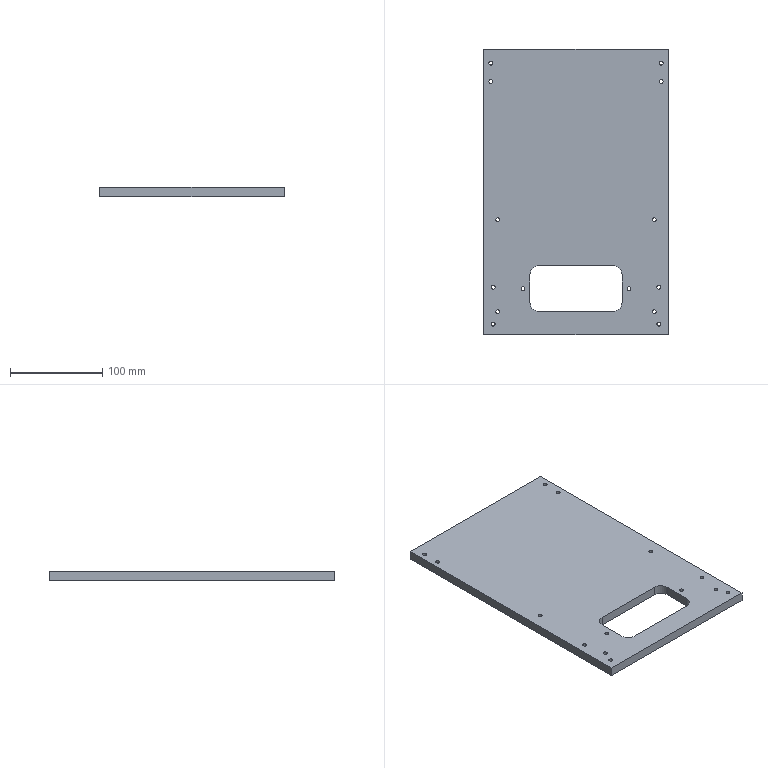Part | SolidWorks | features HoleWzd 4, Cut 1, Extrusion 1, Fillet 1 | 1 solid | 42 faces | box 200 x 310 x 10 mm | volume 568919 mm3 | cylinder 32 | plane 10 | commonest cylinder face diameters 4.2 x28 20 x4
STEP:
#1=CARTESIAN_POINT('',(-87.9,-143.5,5.));
#2=VERTEX_POINT('',#1);
#3=CARTESIAN_POINT('',(-92.1,-143.5,5.));
#4=VERTEX_POINT('',#3);
#5=CARTESIAN_POINT('',(-90.,-143.5,5.));
#6=DIRECTION('',(0.,0.,-1.));
#7=DIRECTION('',(-1.,0.,0.));
#8=AXIS2_PLACEMENT_3D('',#5,#6,#7);
#9=CIRCLE('',#8,2.1);
#10=EDGE_CURVE('',#2,#4,#9,.T.);
#11=ORIENTED_EDGE('',*,*,#10,.F.);
#12=CARTESIAN_POINT('',(-87.9,-143.5,-5.));
#13=VERTEX_POINT('',#12);
#14=CARTESIAN_POINT('',(-87.9,-143.5,-5.));
#15=DIRECTION('',(0.,0.,-1.));
#16=VECTOR('',#15,1000.);
#17=LINE('',#14,#16);
#18=EDGE_CURVE('',#2,#13,#17,.T.);
#19=ORIENTED_EDGE('',*,*,#18,.T.);
#20=CARTESIAN_POINT('',(-92.1,-143.5,-5.));
#21=VERTEX_POINT('',#20);
#22=CARTESIAN_POINT('',(-90.,-143.5,-5.));
#23=DIRECTION('',(0.,0.,-1.));
#24=DIRECTION('',(-1.,0.,0.));
#25=AXIS2_PLACEMENT_3D('',#22,#23,#24);
#26=CIRCLE('',#25,2.1);
#27=EDGE_CURVE('',#13,#21,#26,.T.);
#28=ORIENTED_EDGE('',*,*,#27,.T.);
#29=CARTESIAN_POINT('',(-92.1,-143.5,-5.));
#30=DIRECTION('',(0.,0.,-1.));
#31=VECTOR('',#30,1000.);
#32=LINE('',#29,#31);
#33=EDGE_CURVE('',#4,#21,#32,.T.);
#34=ORIENTED_EDGE('',*,*,#33,.F.);
#35=EDGE_LOOP('',(#11,#19,#28,#34));
#36=FACE_OUTER_BOUND('',#35,.T.);
#37=CARTESIAN_POINT('',(-90.,-143.5,-5.));
#38=DIRECTION('',(0.,0.,-1.));
#39=DIRECTION('',(-1.,0.,0.));
#40=AXIS2_PLACEMENT_3D('',#37,#38,#39);
#41=CYLINDRICAL_SURFACE('',#40,2.1);
#42=ADVANCED_FACE('',(#36),#41,.F.);
#43=CARTESIAN_POINT('',(-87.9,-103.5,5.));
#44=VERTEX_POINT('',#43);
#45=CARTESIAN_POINT('',(-92.1,-103.5,5.));
#46=VERTEX_POINT('',#45);
#47=CARTESIAN_POINT('',(-90.,-103.5,5.));
#48=DIRECTION('',(0.,0.,-1.));
#49=DIRECTION('',(-1.,0.,0.));
#50=AXIS2_PLACEMENT_3D('',#47,#48,#49);
#51=CIRCLE('',#50,2.1);
#52=EDGE_CURVE('',#44,#46,#51,.T.);
#53=ORIENTED_EDGE('',*,*,#52,.F.);
#54=CARTESIAN_POINT('',(-87.9,-103.5,-5.));
#55=VERTEX_POINT('',#54);
#56=CARTESIAN_POINT('',(-87.9,-103.5,-5.));
#57=DIRECTION('',(0.,0.,-1.));
#58=VECTOR('',#57,1000.);
#59=LINE('',#56,#58);
#60=EDGE_CURVE('',#44,#55,#59,.T.);
#61=ORIENTED_EDGE('',*,*,#60,.T.);
#62=CARTESIAN_POINT('',(-92.1,-103.5,-5.));
#63=VERTEX_POINT('',#62);
#64=CARTESIAN_POINT('',(-90.,-103.5,-5.));
#65=DIRECTION('',(0.,0.,-1.));
#66=DIRECTION('',(-1.,0.,0.));
#67=AXIS2_PLACEMENT_3D('',#64,#65,#66);
#68=CIRCLE('',#67,2.1);
#69=EDGE_CURVE('',#55,#63,#68,.T.);
#70=ORIENTED_EDGE('',*,*,#69,.T.);
#71=CARTESIAN_POINT('',(-92.1,-103.5,-5.));
#72=DIRECTION('',(0.,0.,-1.));
#73=VECTOR('',#72,1000.);
#74=LINE('',#71,#73);
#75=EDGE_CURVE('',#46,#63,#74,.T.);
#76=ORIENTED_EDGE('',*,*,#75,.F.);
#77=EDGE_LOOP('',(#53,#61,#70,#76));
#78=FACE_OUTER_BOUND('',#77,.T.);
#79=CARTESIAN_POINT('',(-90.,-103.5,-5.));
#80=DIRECTION('',(0.,0.,-1.));
#81=DIRECTION('',(-1.,0.,0.));
#82=AXIS2_PLACEMENT_3D('',#79,#80,#81);
#83=CYLINDRICAL_SURFACE('',#82,2.1);
#84=ADVANCED_FACE('',(#78),#83,.F.);
#85=CARTESIAN_POINT('',(92.1,-103.5,5.));
#86=VERTEX_POINT('',#85);
#87=CARTESIAN_POINT('',(87.9,-103.5,5.));
#88=VERTEX_POINT('',#87);
#89=CARTESIAN_POINT('',(90.,-103.5,5.));
#90=DIRECTION('',(0.,0.,-1.));
#91=DIRECTION('',(-1.,0.,0.));
#92=AXIS2_PLACEMENT_3D('',#89,#90,#91);
#93=CIRCLE('',#92,2.1);
#94=EDGE_CURVE('',#86,#88,#93,.T.);
#95=ORIENTED_EDGE('',*,*,#94,.F.);
#96=CARTESIAN_POINT('',(92.1,-103.5,-5.));
#97=VERTEX_POINT('',#96);
#98=CARTESIAN_POINT('',(92.1,-103.5,-5.));
#99=DIRECTION('',(0.,0.,-1.));
#100=VECTOR('',#99,1000.);
#101=LINE('',#98,#100);
#102=EDGE_CURVE('',#86,#97,#101,.T.);
#103=ORIENTED_EDGE('',*,*,#102,.T.);
#104=CARTESIAN_POINT('',(87.9,-103.5,-5.));
#105=VERTEX_POINT('',#104);
#106=CARTESIAN_POINT('',(90.,-103.5,-5.));
#107=DIRECTION('',(0.,0.,-1.));
#108=DIRECTION('',(-1.,0.,0.));
#109=AXIS2_PLACEMENT_3D('',#106,#107,#108);
#110=CIRCLE('',#109,2.1);
#111=EDGE_CURVE('',#97,#105,#110,.T.);
#112=ORIENTED_EDGE('',*,*,#111,.T.);
#113=CARTESIAN_POINT('',(87.9,-103.5,-5.));
#114=DIRECTION('',(0.,0.,-1.));
#115=VECTOR('',#114,1000.);
#116=LINE('',#113,#115);
#117=EDGE_CURVE('',#88,#105,#116,.T.);
#118=ORIENTED_EDGE('',*,*,#117,.F.);
#119=EDGE_LOOP('',(#95,#103,#112,#118));
#120=FACE_OUTER_BOUND('',#119,.T.);
#121=CARTESIAN_POINT('',(90.,-103.5,-5.));
#122=DIRECTION('',(0.,0.,-1.));
#123=DIRECTION('',(-1.,0.,0.));
#124=AXIS2_PLACEMENT_3D('',#121,#122,#123);
#125=CYLINDRICAL_SURFACE('',#124,2.1);
#126=ADVANCED_FACE('',(#120),#125,.F.);
#127=CARTESIAN_POINT('',(92.1,-143.5,5.));
#128=VERTEX_POINT('',#127);
#129=CARTESIAN_POINT('',(87.9,-143.5,5.));
#130=VERTEX_POINT('',#129);
#131=CARTESIAN_POINT('',(90.,-143.5,5.));
#132=DIRECTION('',(0.,0.,-1.));
#133=DIRECTION('',(-1.,0.,0.));
#134=AXIS2_PLACEMENT_3D('',#131,#132,#133);
#135=CIRCLE('',#134,2.1);
#136=EDGE_CURVE('',#128,#130,#135,.T.);
#137=ORIENTED_EDGE('',*,*,#136,.F.);
#138=CARTESIAN_POINT('',(92.1,-143.5,-5.));
#139=VERTEX_POINT('',#138);
#140=CARTESIAN_POINT('',(92.1,-143.5,-5.));
#141=DIRECTION('',(0.,0.,-1.));
#142=VECTOR('',#141,1000.);
#143=LINE('',#140,#142);
#144=EDGE_CURVE('',#128,#139,#143,.T.);
#145=ORIENTED_EDGE('',*,*,#144,.T.);
#146=CARTESIAN_POINT('',(87.9,-143.5,-5.));
#147=VERTEX_POINT('',#146);
#148=CARTESIAN_POINT('',(90.,-143.5,-5.));
#149=DIRECTION('',(0.,0.,-1.));
#150=DIRECTION('',(-1.,0.,0.));
#151=AXIS2_PLACEMENT_3D('',#148,#149,#150);
#152=CIRCLE('',#151,2.1);
#153=EDGE_CURVE('',#139,#147,#152,.T.);
#154=ORIENTED_EDGE('',*,*,#153,.T.);
#155=CARTESIAN_POINT('',(87.9,-143.5,-5.));
#156=DIRECTION('',(0.,0.,-1.));
#157=VECTOR('',#156,1000.);
#158=LINE('',#155,#157);
#159=EDGE_CURVE('',#130,#147,#158,.T.);
#160=ORIENTED_EDGE('',*,*,#159,.F.);
#161=EDGE_LOOP('',(#137,#145,#154,#160));
#162=FACE_OUTER_BOUND('',#161,.T.);
#163=CARTESIAN_POINT('',(90.,-143.5,-5.));
#164=DIRECTION('',(0.,0.,-1.));
#165=DIRECTION('',(-1.,0.,0.));
#166=AXIS2_PLACEMENT_3D('',#163,#164,#165);
#167=CYLINDRICAL_SURFACE('',#166,2.1);
#168=ADVANCED_FACE('',(#162),#167,.F.);
#169=CARTESIAN_POINT('',(59.6,-105.,5.));
#170=VERTEX_POINT('',#169);
#171=CARTESIAN_POINT('',(55.4,-105.,5.));
#172=VERTEX_POINT('',#171);
#173=CARTESIAN_POINT('',(57.5,-105.,5.));
#174=DIRECTION('',(0.,0.,-1.));
#175=DIRECTION('',(-1.,0.,0.));
#176=AXIS2_PLACEMENT_3D('',#173,#174,#175);
#177=CIRCLE('',#176,2.1);
#178=EDGE_CURVE('',#170,#172,#177,.T.);
#179=ORIENTED_EDGE('',*,*,#178,.F.);
#180=CARTESIAN_POINT('',(59.6,-105.,-5.));
#181=VERTEX_POINT('',#180);
#182=CARTESIAN_POINT('',(59.6,-105.,-5.));
#183=DIRECTION('',(0.,0.,-1.));
#184=VECTOR('',#183,1000.);
#185=LINE('',#182,#184);
#186=EDGE_CURVE('',#170,#181,#185,.T.);
#187=ORIENTED_EDGE('',*,*,#186,.T.);
#188=CARTESIAN_POINT('',(55.4,-105.,-5.));
#189=VERTEX_POINT('',#188);
#190=CARTESIAN_POINT('',(57.5,-105.,-5.));
#191=DIRECTION('',(0.,0.,-1.));
#192=DIRECTION('',(-1.,0.,0.));
#193=AXIS2_PLACEMENT_3D('',#190,#191,#192);
#194=CIRCLE('',#193,2.1);
#195=EDGE_CURVE('',#181,#189,#194,.T.);
#196=ORIENTED_EDGE('',*,*,#195,.T.);
#197=CARTESIAN_POINT('',(55.4,-105.,-5.));
#198=DIRECTION('',(0.,0.,-1.));
#199=VECTOR('',#198,1000.);
#200=LINE('',#197,#199);
#201=EDGE_CURVE('',#172,#189,#200,.T.);
#202=ORIENTED_EDGE('',*,*,#201,.F.);
#203=EDGE_LOOP('',(#179,#187,#196,#202));
#204=FACE_OUTER_BOUND('',#203,.T.);
#205=CARTESIAN_POINT('',(57.5,-105.,-5.));
#206=DIRECTION('',(0.,0.,-1.));
#207=DIRECTION('',(-1.,0.,0.));
#208=AXIS2_PLACEMENT_3D('',#205,#206,#207);
#209=CYLINDRICAL_SURFACE('',#208,2.1);
#210=ADVANCED_FACE('',(#204),#209,.F.);
#211=CARTESIAN_POINT('',(-55.4,-105.,5.));
#212=VERTEX_POINT('',#211);
#213=CARTESIAN_POINT('',(-59.6,-105.,5.));
#214=VERTEX_POINT('',#213);
#215=CARTESIAN_POINT('',(-57.5,-105.,5.));
#216=DIRECTION('',(0.,0.,-1.));
#217=DIRECTION('',(-1.,0.,0.));
#218=AXIS2_PLACEMENT_3D('',#215,#216,#217);
#219=CIRCLE('',#218,2.1);
#220=EDGE_CURVE('',#212,#214,#219,.T.);
#221=ORIENTED_EDGE('',*,*,#220,.F.);
#222=CARTESIAN_POINT('',(-55.4,-105.,-5.));
#223=VERTEX_POINT('',#222);
#224=CARTESIAN_POINT('',(-55.4,-105.,-5.));
#225=DIRECTION('',(0.,0.,-1.));
#226=VECTOR('',#225,1000.);
#227=LINE('',#224,#226);
#228=EDGE_CURVE('',#212,#223,#227,.T.);
#229=ORIENTED_EDGE('',*,*,#228,.T.);
#230=CARTESIAN_POINT('',(-59.6,-105.,-5.));
#231=VERTEX_POINT('',#230);
#232=CARTESIAN_POINT('',(-57.5,-105.,-5.));
#233=DIRECTION('',(0.,0.,-1.));
#234=DIRECTION('',(-1.,0.,0.));
#235=AXIS2_PLACEMENT_3D('',#232,#233,#234);
#236=CIRCLE('',#235,2.1);
#237=EDGE_CURVE('',#223,#231,#236,.T.);
#238=ORIENTED_EDGE('',*,*,#237,.T.);
#239=CARTESIAN_POINT('',(-59.6,-105.,-5.));
#240=DIRECTION('',(0.,0.,-1.));
#241=VECTOR('',#240,1000.);
#242=LINE('',#239,#241);
#243=EDGE_CURVE('',#214,#231,#242,.T.);
#244=ORIENTED_EDGE('',*,*,#243,.F.);
#245=EDGE_LOOP('',(#221,#229,#238,#244));
#246=FACE_OUTER_BOUND('',#245,.T.);
#247=CARTESIAN_POINT('',(-57.5,-105.,-5.));
#248=DIRECTION('',(0.,0.,-1.));
#249=DIRECTION('',(-1.,0.,0.));
#250=AXIS2_PLACEMENT_3D('',#247,#248,#249);
#251=CYLINDRICAL_SURFACE('',#250,2.1);
#252=ADVANCED_FACE('',(#246),#251,.F.);
#253=CARTESIAN_POINT('',(-90.4,120.,5.));
#254=VERTEX_POINT('',#253);
#255=CARTESIAN_POINT('',(-94.6,120.,5.));
#256=VERTEX_POINT('',#255);
#257=CARTESIAN_POINT('',(-92.5,120.,5.));
#258=DIRECTION('',(0.,0.,-1.));
#259=DIRECTION('',(-1.,0.,0.));
#260=AXIS2_PLACEMENT_3D('',#257,#258,#259);
#261=CIRCLE('',#260,2.1);
#262=EDGE_CURVE('',#254,#256,#261,.T.);
#263=ORIENTED_EDGE('',*,*,#262,.F.);
#264=CARTESIAN_POINT('',(-90.4,120.,-5.));
#265=VERTEX_POINT('',#264);
#266=CARTESIAN_POINT('',(-90.4,120.,-5.));
#267=DIRECTION('',(0.,0.,-1.));
#268=VECTOR('',#267,1000.);
#269=LINE('',#266,#268);
#270=EDGE_CURVE('',#254,#265,#269,.T.);
#271=ORIENTED_EDGE('',*,*,#270,.T.);
#272=CARTESIAN_POINT('',(-94.6,120.,-5.));
#273=VERTEX_POINT('',#272);
#274=CARTESIAN_POINT('',(-92.5,120.,-5.));
#275=DIRECTION('',(0.,0.,-1.));
#276=DIRECTION('',(-1.,0.,0.));
#277=AXIS2_PLACEMENT_3D('',#274,#275,#276);
#278=CIRCLE('',#277,2.1);
#279=EDGE_CURVE('',#265,#273,#278,.T.);
#280=ORIENTED_EDGE('',*,*,#279,.T.);
#281=CARTESIAN_POINT('',(-94.6,120.,-5.));
#282=DIRECTION('',(0.,0.,-1.));
#283=VECTOR('',#282,1000.);
#284=LINE('',#281,#283);
#285=EDGE_CURVE('',#256,#273,#284,.T.);
#286=ORIENTED_EDGE('',*,*,#285,.F.);
#287=EDGE_LOOP('',(#263,#271,#280,#286));
#288=FACE_OUTER_BOUND('',#287,.T.);
#289=CARTESIAN_POINT('',(-92.5,120.,-5.));
#290=DIRECTION('',(0.,0.,-1.));
#291=DIRECTION('',(-1.,0.,0.));
#292=AXIS2_PLACEMENT_3D('',#289,#290,#291);
#293=CYLINDRICAL_SURFACE('',#292,2.1);
#294=ADVANCED_FACE('',(#288),#293,.F.);
#295=CARTESIAN_POINT('',(-90.4,140.,5.));
#296=VERTEX_POINT('',#295);
#297=CARTESIAN_POINT('',(-94.6,140.,5.));
#298=VERTEX_POINT('',#297);
#299=CARTESIAN_POINT('',(-92.5,140.,5.));
#300=DIRECTION('',(0.,0.,-1.));
#301=DIRECTION('',(-1.,0.,0.));
#302=AXIS2_PLACEMENT_3D('',#299,#300,#301);
#303=CIRCLE('',#302,2.1);
#304=EDGE_CURVE('',#296,#298,#303,.T.);
#305=ORIENTED_EDGE('',*,*,#304,.F.);
#306=CARTESIAN_POINT('',(-90.4,140.,-5.));
#307=VERTEX_POINT('',#306);
#308=CARTESIAN_POINT('',(-90.4,140.,-5.));
#309=DIRECTION('',(0.,0.,-1.));
#310=VECTOR('',#309,1000.);
#311=LINE('',#308,#310);
#312=EDGE_CURVE('',#296,#307,#311,.T.);
#313=ORIENTED_EDGE('',*,*,#312,.T.);
#314=CARTESIAN_POINT('',(-94.6,140.,-5.));
#315=VERTEX_POINT('',#314);
#316=CARTESIAN_POINT('',(-92.5,140.,-5.));
#317=DIRECTION('',(0.,0.,-1.));
#318=DIRECTION('',(-1.,0.,0.));
#319=AXIS2_PLACEMENT_3D('',#316,#317,#318);
#320=CIRCLE('',#319,2.1);
#321=EDGE_CURVE('',#307,#315,#320,.T.);
#322=ORIENTED_EDGE('',*,*,#321,.T.);
#323=CARTESIAN_POINT('',(-94.6,140.,-5.));
#324=DIRECTION('',(0.,0.,-1.));
#325=VECTOR('',#324,1000.);
#326=LINE('',#323,#325);
#327=EDGE_CURVE('',#298,#315,#326,.T.);
#328=ORIENTED_EDGE('',*,*,#327,.F.);
#329=EDGE_LOOP('',(#305,#313,#322,#328));
#330=FACE_OUTER_BOUND('',#329,.T.);
#331=CARTESIAN_POINT('',(-92.5,140.,-5.));
#332=DIRECTION('',(0.,0.,-1.));
#333=DIRECTION('',(-1.,0.,0.));
#334=AXIS2_PLACEMENT_3D('',#331,#332,#333);
#335=CYLINDRICAL_SURFACE('',#334,2.1);
#336=ADVANCED_FACE('',(#330),#335,.F.);
#337=CARTESIAN_POINT('',(94.6,140.,5.));
#338=VERTEX_POINT('',#337);
#339=CARTESIAN_POINT('',(90.4,140.,5.));
#340=VERTEX_POINT('',#339);
#341=CARTESIAN_POINT('',(92.5,140.,5.));
#342=DIRECTION('',(0.,0.,-1.));
#343=DIRECTION('',(-1.,0.,0.));
#344=AXIS2_PLACEMENT_3D('',#341,#342,#343);
#345=CIRCLE('',#344,2.1);
#346=EDGE_CURVE('',#338,#340,#345,.T.);
#347=ORIENTED_EDGE('',*,*,#346,.F.);
#348=CARTESIAN_POINT('',(94.6,140.,-5.));
#349=VERTEX_POINT('',#348);
#350=CARTESIAN_POINT('',(94.6,140.,-5.));
#351=DIRECTION('',(0.,0.,-1.));
#352=VECTOR('',#351,1000.);
#353=LINE('',#350,#352);
#354=EDGE_CURVE('',#338,#349,#353,.T.);
#355=ORIENTED_EDGE('',*,*,#354,.T.);
#356=CARTESIAN_POINT('',(90.4,140.,-5.));
#357=VERTEX_POINT('',#356);
#358=CARTESIAN_POINT('',(92.5,140.,-5.));
#359=DIRECTION('',(0.,0.,-1.));
#360=DIRECTION('',(-1.,0.,0.));
#361=AXIS2_PLACEMENT_3D('',#358,#359,#360);
#362=CIRCLE('',#361,2.1);
#363=EDGE_CURVE('',#349,#357,#362,.T.);
#364=ORIENTED_EDGE('',*,*,#363,.T.);
#365=CARTESIAN_POINT('',(90.4,140.,-5.));
#366=DIRECTION('',(0.,0.,-1.));
#367=VECTOR('',#366,1000.);
#368=LINE('',#365,#367);
#369=EDGE_CURVE('',#340,#357,#368,.T.);
#370=ORIENTED_EDGE('',*,*,#369,.F.);
#371=EDGE_LOOP('',(#347,#355,#364,#370));
#372=FACE_OUTER_BOUND('',#371,.T.);
#373=CARTESIAN_POINT('',(92.5,140.,-5.));
#374=DIRECTION('',(0.,0.,-1.));
#375=DIRECTION('',(-1.,0.,0.));
#376=AXIS2_PLACEMENT_3D('',#373,#374,#375);
#377=CYLINDRICAL_SURFACE('',#376,2.1);
#378=ADVANCED_FACE('',(#372),#377,.F.);
#379=CARTESIAN_POINT('',(94.6,120.,5.));
#380=VERTEX_POINT('',#379);
#381=CARTESIAN_POINT('',(90.4,120.,5.));
#382=VERTEX_POINT('',#381);
#383=CARTESIAN_POINT('',(92.5,120.,5.));
#384=DIRECTION('',(0.,0.,-1.));
#385=DIRECTION('',(-1.,0.,0.));
#386=AXIS2_PLACEMENT_3D('',#383,#384,#385);
#387=CIRCLE('',#386,2.1);
#388=EDGE_CURVE('',#380,#382,#387,.T.);
#389=ORIENTED_EDGE('',*,*,#388,.F.);
#390=CARTESIAN_POINT('',(94.6,120.,-5.));
#391=VERTEX_POINT('',#390);
#392=CARTESIAN_POINT('',(94.6,120.,-5.));
#393=DIRECTION('',(0.,0.,-1.));
#394=VECTOR('',#393,1000.);
#395=LINE('',#392,#394);
#396=EDGE_CURVE('',#380,#391,#395,.T.);
#397=ORIENTED_EDGE('',*,*,#396,.T.);
#398=CARTESIAN_POINT('',(90.4,120.,-5.));
#399=VERTEX_POINT('',#398);
#400=CARTESIAN_POINT('',(92.5,120.,-5.));
#401=DIRECTION('',(0.,0.,-1.));
#402=DIRECTION('',(-1.,0.,0.));
#403=AXIS2_PLACEMENT_3D('',#400,#401,#402);
#404=CIRCLE('',#403,2.1);
#405=EDGE_CURVE('',#391,#399,#404,.T.);
#406=ORIENTED_EDGE('',*,*,#405,.T.);
#407=CARTESIAN_POINT('',(90.4,120.,-5.));
#408=DIRECTION('',(0.,0.,-1.));
#409=VECTOR('',#408,1000.);
#410=LINE('',#407,#409);
#411=EDGE_CURVE('',#382,#399,#410,.T.);
#412=ORIENTED_EDGE('',*,*,#411,.F.);
#413=EDGE_LOOP('',(#389,#397,#406,#412));
#414=FACE_OUTER_BOUND('',#413,.T.);
#415=CARTESIAN_POINT('',(92.5,120.,-5.));
#416=DIRECTION('',(0.,0.,-1.));
#417=DIRECTION('',(-1.,0.,0.));
#418=AXIS2_PLACEMENT_3D('',#415,#416,#417);
#419=CYLINDRICAL_SURFACE('',#418,2.1);
#420=ADVANCED_FACE('',(#414),#419,.F.);
#421=CARTESIAN_POINT('',(82.9,-130.,-5.));
#422=VERTEX_POINT('',#421);
#423=CARTESIAN_POINT('',(87.1,-130.,-5.));
#424=VERTEX_POINT('',#423);
#425=CARTESIAN_POINT('',(85.,-130.,-5.));
#426=DIRECTION('',(0.,0.,1.));
#427=DIRECTION('',(1.,0.,0.));
#428=AXIS2_PLACEMENT_3D('',#425,#426,#427);
#429=CIRCLE('',#428,2.1);
#430=EDGE_CURVE('',#422,#424,#429,.T.);
#431=ORIENTED_EDGE('',*,*,#430,.F.);
#432=CARTESIAN_POINT('',(82.9,-130.,5.));
#433=VERTEX_POINT('',#432);
#434=CARTESIAN_POINT('',(82.9,-130.,5.));
#435=DIRECTION('',(0.,0.,1.));
#436=VECTOR('',#435,1000.);
#437=LINE('',#434,#436);
#438=EDGE_CURVE('',#422,#433,#437,.T.);
#439=ORIENTED_EDGE('',*,*,#438,.T.);
#440=CARTESIAN_POINT('',(87.1,-130.,5.));
#441=VERTEX_POINT('',#440);
#442=CARTESIAN_POINT('',(85.,-130.,5.));
#443=DIRECTION('',(0.,0.,1.));
#444=DIRECTION('',(1.,0.,0.));
#445=AXIS2_PLACEMENT_3D('',#442,#443,#444);
#446=CIRCLE('',#445,2.1);
#447=EDGE_CURVE('',#433,#441,#446,.T.);
#448=ORIENTED_EDGE('',*,*,#447,.T.);
#449=CARTESIAN_POINT('',(87.1,-130.,5.));
#450=DIRECTION('',(0.,0.,1.));
#451=VECTOR('',#450,1000.);
#452=LINE('',#449,#451);
#453=EDGE_CURVE('',#424,#441,#452,.T.);
#454=ORIENTED_EDGE('',*,*,#453,.F.);
#455=EDGE_LOOP('',(#431,#439,#448,#454));
#456=FACE_OUTER_BOUND('',#455,.T.);
#457=CARTESIAN_POINT('',(85.,-130.,5.));
#458=DIRECTION('',(0.,0.,1.));
#459=DIRECTION('',(1.,0.,0.));
#460=AXIS2_PLACEMENT_3D('',#457,#458,#459);
#461=CYLINDRICAL_SURFACE('',#460,2.1);
#462=ADVANCED_FACE('',(#456),#461,.F.);
#463=CARTESIAN_POINT('',(82.9,-30.,-5.));
#464=VERTEX_POINT('',#463);
#465=CARTESIAN_POINT('',(87.1,-30.,-5.));
#466=VERTEX_POINT('',#465);
#467=CARTESIAN_POINT('',(85.,-30.,-5.));
#468=DIRECTION('',(0.,0.,1.));
#469=DIRECTION('',(1.,0.,0.));
#470=AXIS2_PLACEMENT_3D('',#467,#468,#469);
#471=CIRCLE('',#470,2.1);
#472=EDGE_CURVE('',#464,#466,#471,.T.);
#473=ORIENTED_EDGE('',*,*,#472,.F.);
#474=CARTESIAN_POINT('',(82.9,-30.,5.));
#475=VERTEX_POINT('',#474);
#476=CARTESIAN_POINT('',(82.9,-30.,5.));
#477=DIRECTION('',(0.,0.,1.));
#478=VECTOR('',#477,1000.);
#479=LINE('',#476,#478);
#480=EDGE_CURVE('',#464,#475,#479,.T.);
#481=ORIENTED_EDGE('',*,*,#480,.T.);
#482=CARTESIAN_POINT('',(87.1,-30.,5.));
#483=VERTEX_POINT('',#482);
#484=CARTESIAN_POINT('',(85.,-30.,5.));
#485=DIRECTION('',(0.,0.,1.));
#486=DIRECTION('',(1.,0.,0.));
#487=AXIS2_PLACEMENT_3D('',#484,#485,#486);
#488=CIRCLE('',#487,2.1);
#489=EDGE_CURVE('',#475,#483,#488,.T.);
#490=ORIENTED_EDGE('',*,*,#489,.T.);
#491=CARTESIAN_POINT('',(87.1,-30.,5.));
#492=DIRECTION('',(0.,0.,1.));
#493=VECTOR('',#492,1000.);
#494=LINE('',#491,#493);
#495=EDGE_CURVE('',#466,#483,#494,.T.);
#496=ORIENTED_EDGE('',*,*,#495,.F.);
#497=EDGE_LOOP('',(#473,#481,#490,#496));
#498=FACE_OUTER_BOUND('',#497,.T.);
#499=CARTESIAN_POINT('',(85.,-30.,5.));
#500=DIRECTION('',(0.,0.,1.));
#501=DIRECTION('',(1.,0.,0.));
#502=AXIS2_PLACEMENT_3D('',#499,#500,#501);
#503=CYLINDRICAL_SURFACE('',#502,2.1);
#504=ADVANCED_FACE('',(#498),#503,.F.);
#505=CARTESIAN_POINT('',(-87.1,-30.,-5.));
#506=VERTEX_POINT('',#505);
#507=CARTESIAN_POINT('',(-82.9,-30.,-5.));
#508=VERTEX_POINT('',#507);
#509=CARTESIAN_POINT('',(-85.,-30.,-5.));
#510=DIRECTION('',(0.,0.,1.));
#511=DIRECTION('',(1.,0.,0.));
#512=AXIS2_PLACEMENT_3D('',#509,#510,#511);
#513=CIRCLE('',#512,2.1);
#514=EDGE_CURVE('',#506,#508,#513,.T.);
#515=ORIENTED_EDGE('',*,*,#514,.F.);
#516=CARTESIAN_POINT('',(-87.1,-30.,5.));
#517=VERTEX_POINT('',#516);
#518=CARTESIAN_POINT('',(-87.1,-30.,5.));
#519=DIRECTION('',(0.,0.,1.));
#520=VECTOR('',#519,1000.);
#521=LINE('',#518,#520);
#522=EDGE_CURVE('',#506,#517,#521,.T.);
#523=ORIENTED_EDGE('',*,*,#522,.T.);
#524=CARTESIAN_POINT('',(-82.9,-30.,5.));
#525=VERTEX_POINT('',#524);
#526=CARTESIAN_POINT('',(-85.,-30.,5.));
#527=DIRECTION('',(0.,0.,1.));
#528=DIRECTION('',(1.,0.,0.));
#529=AXIS2_PLACEMENT_3D('',#526,#527,#528);
#530=CIRCLE('',#529,2.1);
#531=EDGE_CURVE('',#517,#525,#530,.T.);
#532=ORIENTED_EDGE('',*,*,#531,.T.);
#533=CARTESIAN_POINT('',(-82.9,-30.,5.));
#534=DIRECTION('',(0.,0.,1.));
#535=VECTOR('',#534,1000.);
#536=LINE('',#533,#535);
#537=EDGE_CURVE('',#508,#525,#536,.T.);
#538=ORIENTED_EDGE('',*,*,#537,.F.);
#539=EDGE_LOOP('',(#515,#523,#532,#538));
#540=FACE_OUTER_BOUND('',#539,.T.);
#541=CARTESIAN_POINT('',(-85.,-30.,5.));
#542=DIRECTION('',(0.,0.,1.));
#543=DIRECTION('',(1.,0.,0.));
#544=AXIS2_PLACEMENT_3D('',#541,#542,#543);
#545=CYLINDRICAL_SURFACE('',#544,2.1);
#546=ADVANCED_FACE('',(#540),#545,.F.);
#547=CARTESIAN_POINT('',(-87.1,-130.,-5.));
#548=VERTEX_POINT('',#547);
#549=CARTESIAN_POINT('',(-82.9,-130.,-5.));
#550=VERTEX_POINT('',#549);
#551=CARTESIAN_POINT('',(-85.,-130.,-5.));
#552=DIRECTION('',(0.,0.,1.));
#553=DIRECTION('',(1.,0.,0.));
#554=AXIS2_PLACEMENT_3D('',#551,#552,#553);
#555=CIRCLE('',#554,2.1);
#556=EDGE_CURVE('',#548,#550,#555,.T.);
#557=ORIENTED_EDGE('',*,*,#556,.F.);
#558=CARTESIAN_POINT('',(-87.1,-130.,5.));
#559=VERTEX_POINT('',#558);
#560=CARTESIAN_POINT('',(-87.1,-130.,5.));
#561=DIRECTION('',(0.,0.,1.));
#562=VECTOR('',#561,1000.);
#563=LINE('',#560,#562);
#564=EDGE_CURVE('',#548,#559,#563,.T.);
#565=ORIENTED_EDGE('',*,*,#564,.T.);
#566=CARTESIAN_POINT('',(-82.9,-130.,5.));
#567=VERTEX_POINT('',#566);
#568=CARTESIAN_POINT('',(-85.,-130.,5.));
#569=DIRECTION('',(0.,0.,1.));
#570=DIRECTION('',(1.,0.,0.));
#571=AXIS2_PLACEMENT_3D('',#568,#569,#570);
#572=CIRCLE('',#571,2.1);
#573=EDGE_CURVE('',#559,#567,#572,.T.);
#574=ORIENTED_EDGE('',*,*,#573,.T.);
#575=CARTESIAN_POINT('',(-82.9,-130.,5.));
#576=DIRECTION('',(0.,0.,1.));
#577=VECTOR('',#576,1000.);
#578=LINE('',#575,#577);
#579=EDGE_CURVE('',#550,#567,#578,.T.);
#580=ORIENTED_EDGE('',*,*,#579,.F.);
#581=EDGE_LOOP('',(#557,#565,#574,#580));
#582=FACE_OUTER_BOUND('',#581,.T.);
#583=CARTESIAN_POINT('',(-85.,-130.,5.));
#584=DIRECTION('',(0.,0.,1.));
#585=DIRECTION('',(1.,0.,0.));
#586=AXIS2_PLACEMENT_3D('',#583,#584,#585);
#587=CYLINDRICAL_SURFACE('',#586,2.1);
#588=ADVANCED_FACE('',(#582),#587,.F.);
#589=CARTESIAN_POINT('',(100.,-155.,-5.));
#590=VERTEX_POINT('',#589);
#591=CARTESIAN_POINT('',(100.,155.,-5.));
#592=VERTEX_POINT('',#591);
#593=CARTESIAN_POINT('',(100.,-155.,-5.));
#594=DIRECTION('',(0.,1.,0.));
#595=VECTOR('',#594,1000.);
#596=LINE('',#593,#595);
#597=EDGE_CURVE('',#590,#592,#596,.T.);
#598=ORIENTED_EDGE('',*,*,#597,.T.);
#599=CARTESIAN_POINT('',(100.,155.,5.));
#600=VERTEX_POINT('',#599);
#601=CARTESIAN_POINT('',(100.,155.,5.));
#602=DIRECTION('',(0.,0.,-1.));
#603=VECTOR('',#602,1000.);
#604=LINE('',#601,#603);
#605=EDGE_CURVE('',#600,#592,#604,.T.);
#606=ORIENTED_EDGE('',*,*,#605,.F.);
#607=CARTESIAN_POINT('',(100.,-155.,5.));
#608=VERTEX_POINT('',#607);
#609=CARTESIAN_POINT('',(100.,-155.,5.));
#610=DIRECTION('',(0.,1.,0.));
#611=VECTOR('',#610,1000.);
#612=LINE('',#609,#611);
#613=EDGE_CURVE('',#608,#600,#612,.T.);
#614=ORIENTED_EDGE('',*,*,#613,.F.);
#615=CARTESIAN_POINT('',(100.,-155.,5.));
#616=DIRECTION('',(0.,0.,-1.));
#617=VECTOR('',#616,1000.);
#618=LINE('',#615,#617);
#619=EDGE_CURVE('',#608,#590,#618,.T.);
#620=ORIENTED_EDGE('',*,*,#619,.T.);
#621=EDGE_LOOP('',(#598,#606,#614,#620));
#622=FACE_OUTER_BOUND('',#621,.T.);
#623=CARTESIAN_POINT('',(100.,-155.,5.));
#624=DIRECTION('',(-1.,0.,0.));
#625=DIRECTION('',(0.,0.,1.));
#626=AXIS2_PLACEMENT_3D('',#623,#624,#625);
#627=PLANE('',#626);
#628=ADVANCED_FACE('',(#622),#627,.F.);
#629=CARTESIAN_POINT('',(-100.,155.,-5.));
#630=VERTEX_POINT('',#629);
#631=CARTESIAN_POINT('',(-100.,155.,-5.));
#632=DIRECTION('',(-1.,0.,0.));
#633=VECTOR('',#632,1000.);
#634=LINE('',#631,#633);
#635=EDGE_CURVE('',#592,#630,#634,.T.);
#636=ORIENTED_EDGE('',*,*,#635,.T.);
#637=CARTESIAN_POINT('',(-100.,155.,5.));
#638=VERTEX_POINT('',#637);
#639=CARTESIAN_POINT('',(-100.,155.,5.));
#640=DIRECTION('',(0.,0.,-1.));
#641=VECTOR('',#640,1000.);
#642=LINE('',#639,#641);
#643=EDGE_CURVE('',#638,#630,#642,.T.);
#644=ORIENTED_EDGE('',*,*,#643,.F.);
#645=CARTESIAN_POINT('',(-100.,155.,5.));
#646=DIRECTION('',(-1.,0.,0.));
#647=VECTOR('',#646,1000.);
#648=LINE('',#645,#647);
#649=EDGE_CURVE('',#600,#638,#648,.T.);
#650=ORIENTED_EDGE('',*,*,#649,.F.);
#651=ORIENTED_EDGE('',*,*,#605,.T.);
#652=EDGE_LOOP('',(#636,#644,#650,#651));
#653=FACE_OUTER_BOUND('',#652,.T.);
#654=CARTESIAN_POINT('',(-100.,155.,5.));
#655=DIRECTION('',(0.,-1.,0.));
#656=DIRECTION('',(0.,0.,-1.));
#657=AXIS2_PLACEMENT_3D('',#654,#655,#656);
#658=PLANE('',#657);
#659=ADVANCED_FACE('',(#653),#658,.F.);
#660=CARTESIAN_POINT('',(-100.,-155.,-5.));
#661=VERTEX_POINT('',#660);
#662=CARTESIAN_POINT('',(-100.,-155.,-5.));
#663=DIRECTION('',(0.,-1.,0.));
#664=VECTOR('',#663,1000.);
#665=LINE('',#662,#664);
#666=EDGE_CURVE('',#630,#661,#665,.T.);
#667=ORIENTED_EDGE('',*,*,#666,.T.);
#668=CARTESIAN_POINT('',(-100.,-155.,5.));
#669=VERTEX_POINT('',#668);
#670=CARTESIAN_POINT('',(-100.,-155.,5.));
#671=DIRECTION('',(0.,0.,-1.));
#672=VECTOR('',#671,1000.);
#673=LINE('',#670,#672);
#674=EDGE_CURVE('',#669,#661,#673,.T.);
#675=ORIENTED_EDGE('',*,*,#674,.F.);
#676=CARTESIAN_POINT('',(-100.,-155.,5.));
#677=DIRECTION('',(0.,-1.,0.));
#678=VECTOR('',#677,1000.);
#679=LINE('',#676,#678);
#680=EDGE_CURVE('',#638,#669,#679,.T.);
#681=ORIENTED_EDGE('',*,*,#680,.F.);
#682=ORIENTED_EDGE('',*,*,#643,.T.);
#683=EDGE_LOOP('',(#667,#675,#681,#682));
#684=FACE_OUTER_BOUND('',#683,.T.);
#685=CARTESIAN_POINT('',(-100.,-155.,5.));
#686=DIRECTION('',(1.,0.,0.));
#687=DIRECTION('',(0.,0.,-1.));
#688=AXIS2_PLACEMENT_3D('',#685,#686,#687);
#689=PLANE('',#688);
#690=ADVANCED_FACE('',(#684),#689,.F.);
#691=CARTESIAN_POINT('',(-100.,-155.,-5.));
#692=DIRECTION('',(1.,0.,0.));
#693=VECTOR('',#692,1000.);
#694=LINE('',#691,#693);
#695=EDGE_CURVE('',#661,#590,#694,.T.);
#696=ORIENTED_EDGE('',*,*,#695,.T.);
#697=ORIENTED_EDGE('',*,*,#619,.F.);
#698=CARTESIAN_POINT('',(-100.,-155.,5.));
#699=DIRECTION('',(1.,0.,0.));
#700=VECTOR('',#699,1000.);
#701=LINE('',#698,#700);
#702=EDGE_CURVE('',#669,#608,#701,.T.);
#703=ORIENTED_EDGE('',*,*,#702,.F.);
#704=ORIENTED_EDGE('',*,*,#674,.T.);
#705=EDGE_LOOP('',(#696,#697,#703,#704));
#706=FACE_OUTER_BOUND('',#705,.T.);
#707=CARTESIAN_POINT('',(-100.,-155.,5.));
#708=DIRECTION('',(0.,1.,0.));
#709=DIRECTION('',(0.,0.,1.));
#710=AXIS2_PLACEMENT_3D('',#707,#708,#709);
#711=PLANE('',#710);
#712=ADVANCED_FACE('',(#706),#711,.F.);
#713=CARTESIAN_POINT('',(-90.,-143.5,5.));
#714=DIRECTION('',(0.,0.,-1.));
#715=DIRECTION('',(-1.,0.,0.));
#716=AXIS2_PLACEMENT_3D('',#713,#714,#715);
#717=CIRCLE('',#716,2.1);
#718=EDGE_CURVE('',#4,#2,#717,.T.);
#719=ORIENTED_EDGE('',*,*,#718,.T.);
#720=ORIENTED_EDGE('',*,*,#10,.T.);
#721=EDGE_LOOP('',(#719,#720));
#722=FACE_BOUND('',#721,.T.);
#723=CARTESIAN_POINT('',(-90.,-103.5,5.));
#724=DIRECTION('',(0.,0.,-1.));
#725=DIRECTION('',(-1.,0.,0.));
#726=AXIS2_PLACEMENT_3D('',#723,#724,#725);
#727=CIRCLE('',#726,2.1);
#728=EDGE_CURVE('',#46,#44,#727,.T.);
#729=ORIENTED_EDGE('',*,*,#728,.T.);
#730=ORIENTED_EDGE('',*,*,#52,.T.);
#731=EDGE_LOOP('',(#729,#730));
#732=FACE_BOUND('',#731,.T.);
#733=CARTESIAN_POINT('',(90.,-103.5,5.));
#734=DIRECTION('',(0.,0.,-1.));
#735=DIRECTION('',(-1.,0.,0.));
#736=AXIS2_PLACEMENT_3D('',#733,#734,#735);
#737=CIRCLE('',#736,2.1);
#738=EDGE_CURVE('',#88,#86,#737,.T.);
#739=ORIENTED_EDGE('',*,*,#738,.T.);
#740=ORIENTED_EDGE('',*,*,#94,.T.);
#741=EDGE_LOOP('',(#739,#740));
#742=FACE_BOUND('',#741,.T.);
#743=CARTESIAN_POINT('',(90.,-143.5,5.));
#744=DIRECTION('',(0.,0.,-1.));
#745=DIRECTION('',(-1.,0.,0.));
#746=AXIS2_PLACEMENT_3D('',#743,#744,#745);
#747=CIRCLE('',#746,2.1);
#748=EDGE_CURVE('',#130,#128,#747,.T.);
#749=ORIENTED_EDGE('',*,*,#748,.T.);
#750=ORIENTED_EDGE('',*,*,#136,.T.);
#751=EDGE_LOOP('',(#749,#750));
#752=FACE_BOUND('',#751,.T.);
#753=CARTESIAN_POINT('',(57.5,-105.,5.));
#754=DIRECTION('',(0.,0.,-1.));
#755=DIRECTION('',(-1.,0.,0.));
#756=AXIS2_PLACEMENT_3D('',#753,#754,#755);
#757=CIRCLE('',#756,2.1);
#758=EDGE_CURVE('',#172,#170,#757,.T.);
#759=ORIENTED_EDGE('',*,*,#758,.T.);
#760=ORIENTED_EDGE('',*,*,#178,.T.);
#761=EDGE_LOOP('',(#759,#760));
#762=FACE_BOUND('',#761,.T.);
#763=CARTESIAN_POINT('',(-57.5,-105.,5.));
#764=DIRECTION('',(0.,0.,-1.));
#765=DIRECTION('',(-1.,0.,0.));
#766=AXIS2_PLACEMENT_3D('',#763,#764,#765);
#767=CIRCLE('',#766,2.1);
#768=EDGE_CURVE('',#214,#212,#767,.T.);
#769=ORIENTED_EDGE('',*,*,#768,.T.);
#770=ORIENTED_EDGE('',*,*,#220,.T.);
#771=EDGE_LOOP('',(#769,#770));
#772=FACE_BOUND('',#771,.T.);
#773=CARTESIAN_POINT('',(-92.5,120.,5.));
#774=DIRECTION('',(0.,0.,-1.));
#775=DIRECTION('',(-1.,0.,0.));
#776=AXIS2_PLACEMENT_3D('',#773,#774,#775);
#777=CIRCLE('',#776,2.1);
#778=EDGE_CURVE('',#256,#254,#777,.T.);
#779=ORIENTED_EDGE('',*,*,#778,.T.);
#780=ORIENTED_EDGE('',*,*,#262,.T.);
#781=EDGE_LOOP('',(#779,#780));
#782=FACE_BOUND('',#781,.T.);
#783=CARTESIAN_POINT('',(-92.5,140.,5.));
#784=DIRECTION('',(0.,0.,-1.));
#785=DIRECTION('',(-1.,0.,0.));
#786=AXIS2_PLACEMENT_3D('',#783,#784,#785);
#787=CIRCLE('',#786,2.1);
#788=EDGE_CURVE('',#298,#296,#787,.T.);
#789=ORIENTED_EDGE('',*,*,#788,.T.);
#790=ORIENTED_EDGE('',*,*,#304,.T.);
#791=EDGE_LOOP('',(#789,#790));
#792=FACE_BOUND('',#791,.T.);
#793=CARTESIAN_POINT('',(92.5,140.,5.));
#794=DIRECTION('',(0.,0.,-1.));
#795=DIRECTION('',(-1.,0.,0.));
#796=AXIS2_PLACEMENT_3D('',#793,#794,#795);
#797=CIRCLE('',#796,2.1);
#798=EDGE_CURVE('',#340,#338,#797,.T.);
#799=ORIENTED_EDGE('',*,*,#798,.T.);
#800=ORIENTED_EDGE('',*,*,#346,.T.);
#801=EDGE_LOOP('',(#799,#800));
#802=FACE_BOUND('',#801,.T.);
#803=CARTESIAN_POINT('',(92.5,120.,5.));
#804=DIRECTION('',(0.,0.,-1.));
#805=DIRECTION('',(-1.,0.,0.));
#806=AXIS2_PLACEMENT_3D('',#803,#804,#805);
#807=CIRCLE('',#806,2.1);
#808=EDGE_CURVE('',#382,#380,#807,.T.);
#809=ORIENTED_EDGE('',*,*,#808,.T.);
#810=ORIENTED_EDGE('',*,*,#388,.T.);
#811=EDGE_LOOP('',(#809,#810));
#812=FACE_BOUND('',#811,.T.);
#813=CARTESIAN_POINT('',(85.,-130.,5.));
#814=DIRECTION('',(0.,0.,1.));
#815=DIRECTION('',(1.,0.,0.));
#816=AXIS2_PLACEMENT_3D('',#813,#814,#815);
#817=CIRCLE('',#816,2.1);
#818=EDGE_CURVE('',#441,#433,#817,.T.);
#819=ORIENTED_EDGE('',*,*,#818,.F.);
#820=ORIENTED_EDGE('',*,*,#447,.F.);
#821=EDGE_LOOP('',(#819,#820));
#822=FACE_BOUND('',#821,.T.);
#823=CARTESIAN_POINT('',(85.,-30.,5.));
#824=DIRECTION('',(0.,0.,1.));
#825=DIRECTION('',(1.,0.,0.));
#826=AXIS2_PLACEMENT_3D('',#823,#824,#825);
#827=CIRCLE('',#826,2.1);
#828=EDGE_CURVE('',#483,#475,#827,.T.);
#829=ORIENTED_EDGE('',*,*,#828,.F.);
#830=ORIENTED_EDGE('',*,*,#489,.F.);
#831=EDGE_LOOP('',(#829,#830));
#832=FACE_BOUND('',#831,.T.);
#833=CARTESIAN_POINT('',(-85.,-30.,5.));
#834=DIRECTION('',(0.,0.,1.));
#835=DIRECTION('',(1.,0.,0.));
#836=AXIS2_PLACEMENT_3D('',#833,#834,#835);
#837=CIRCLE('',#836,2.1);
#838=EDGE_CURVE('',#525,#517,#837,.T.);
#839=ORIENTED_EDGE('',*,*,#838,.F.);
#840=ORIENTED_EDGE('',*,*,#531,.F.);
#841=EDGE_LOOP('',(#839,#840));
#842=FACE_BOUND('',#841,.T.);
#843=CARTESIAN_POINT('',(-85.,-130.,5.));
#844=DIRECTION('',(0.,0.,1.));
#845=DIRECTION('',(1.,0.,0.));
#846=AXIS2_PLACEMENT_3D('',#843,#844,#845);
#847=CIRCLE('',#846,2.1);
#848=EDGE_CURVE('',#567,#559,#847,.T.);
#849=ORIENTED_EDGE('',*,*,#848,.F.);
#850=ORIENTED_EDGE('',*,*,#573,.F.);
#851=EDGE_LOOP('',(#849,#850));
#852=FACE_BOUND('',#851,.T.);
#853=CARTESIAN_POINT('',(40.,-80.,5.));
#854=VERTEX_POINT('',#853);
#855=CARTESIAN_POINT('',(-40.,-80.,5.));
#856=VERTEX_POINT('',#855);
#857=CARTESIAN_POINT('',(50.,-80.,5.));
#858=DIRECTION('',(-1.,0.,0.));
#859=VECTOR('',#858,1000.);
#860=LINE('',#857,#859);
#861=EDGE_CURVE('',#854,#856,#860,.T.);
#862=ORIENTED_EDGE('',*,*,#861,.F.);
#863=CARTESIAN_POINT('',(50.,-90.,5.));
#864=VERTEX_POINT('',#863);
#865=CARTESIAN_POINT('',(40.,-90.,5.));
#866=DIRECTION('',(0.,0.,-1.));
#867=DIRECTION('',(-1.,0.,0.));
#868=AXIS2_PLACEMENT_3D('',#865,#866,#867);
#869=CIRCLE('',#868,10.);
#870=EDGE_CURVE('',#854,#864,#869,.T.);
#871=ORIENTED_EDGE('',*,*,#870,.T.);
#872=CARTESIAN_POINT('',(50.,-120.,5.));
#873=VERTEX_POINT('',#872);
#874=CARTESIAN_POINT('',(50.,-130.,5.));
#875=DIRECTION('',(0.,1.,0.));
#876=VECTOR('',#875,1000.);
#877=LINE('',#874,#876);
#878=EDGE_CURVE('',#873,#864,#877,.T.);
#879=ORIENTED_EDGE('',*,*,#878,.F.);
#880=CARTESIAN_POINT('',(40.,-130.,5.));
#881=VERTEX_POINT('',#880);
#882=CARTESIAN_POINT('',(40.,-120.,5.));
#883=DIRECTION('',(0.,0.,-1.));
#884=DIRECTION('',(-1.,0.,0.));
#885=AXIS2_PLACEMENT_3D('',#882,#883,#884);
#886=CIRCLE('',#885,10.);
#887=EDGE_CURVE('',#873,#881,#886,.T.);
#888=ORIENTED_EDGE('',*,*,#887,.T.);
#889=CARTESIAN_POINT('',(-40.,-130.,5.));
#890=VERTEX_POINT('',#889);
#891=CARTESIAN_POINT('',(50.,-130.,5.));
#892=DIRECTION('',(1.,0.,0.));
#893=VECTOR('',#892,1000.);
#894=LINE('',#891,#893);
#895=EDGE_CURVE('',#890,#881,#894,.T.);
#896=ORIENTED_EDGE('',*,*,#895,.F.);
#897=CARTESIAN_POINT('',(-50.,-120.,5.));
#898=VERTEX_POINT('',#897);
#899=CARTESIAN_POINT('',(-40.,-120.,5.));
#900=DIRECTION('',(0.,0.,-1.));
#901=DIRECTION('',(-1.,0.,0.));
#902=AXIS2_PLACEMENT_3D('',#899,#900,#901);
#903=CIRCLE('',#902,10.);
#904=EDGE_CURVE('',#890,#898,#903,.T.);
#905=ORIENTED_EDGE('',*,*,#904,.T.);
#906=CARTESIAN_POINT('',(-50.,-90.,5.));
#907=VERTEX_POINT('',#906);
#908=CARTESIAN_POINT('',(-50.,-130.,5.));
#909=DIRECTION('',(0.,-1.,0.));
#910=VECTOR('',#909,1000.);
#911=LINE('',#908,#910);
#912=EDGE_CURVE('',#907,#898,#911,.T.);
#913=ORIENTED_EDGE('',*,*,#912,.F.);
#914=CARTESIAN_POINT('',(-40.,-90.,5.));
#915=DIRECTION('',(0.,0.,-1.));
#916=DIRECTION('',(-1.,0.,0.));
#917=AXIS2_PLACEMENT_3D('',#914,#915,#916);
#918=CIRCLE('',#917,10.);
#919=EDGE_CURVE('',#907,#856,#918,.T.);
#920=ORIENTED_EDGE('',*,*,#919,.T.);
#921=EDGE_LOOP('',(#862,#871,#879,#888,#896,#905,#913,#920));
#922=FACE_BOUND('',#921,.T.);
#923=ORIENTED_EDGE('',*,*,#613,.T.);
#924=ORIENTED_EDGE('',*,*,#649,.T.);
#925=ORIENTED_EDGE('',*,*,#680,.T.);
#926=ORIENTED_EDGE('',*,*,#702,.T.);
#927=EDGE_LOOP('',(#923,#924,#925,#926));
#928=FACE_OUTER_BOUND('',#927,.T.);
#929=CARTESIAN_POINT('',(0.,0.,5.));
#930=DIRECTION('',(0.,0.,-1.));
#931=DIRECTION('',(-1.,0.,0.));
#932=AXIS2_PLACEMENT_3D('',#929,#930,#931);
#933=PLANE('',#932);
#934=ADVANCED_FACE('',(#722,#732,#742,#752,#762,#772,#782,#792,#802,#812,#822,#832,#842,#852,#922,#928),#933,.F.);
#935=CARTESIAN_POINT('',(-90.,-143.5,-5.));
#936=DIRECTION('',(0.,0.,-1.));
#937=DIRECTION('',(-1.,0.,0.));
#938=AXIS2_PLACEMENT_3D('',#935,#936,#937);
#939=CIRCLE('',#938,2.1);
#940=EDGE_CURVE('',#21,#13,#939,.T.);
#941=ORIENTED_EDGE('',*,*,#940,.F.);
#942=ORIENTED_EDGE('',*,*,#27,.F.);
#943=EDGE_LOOP('',(#941,#942));
#944=FACE_BOUND('',#943,.T.);
#945=CARTESIAN_POINT('',(-90.,-103.5,-5.));
#946=DIRECTION('',(0.,0.,-1.));
#947=DIRECTION('',(-1.,0.,0.));
#948=AXIS2_PLACEMENT_3D('',#945,#946,#947);
#949=CIRCLE('',#948,2.1);
#950=EDGE_CURVE('',#63,#55,#949,.T.);
#951=ORIENTED_EDGE('',*,*,#950,.F.);
#952=ORIENTED_EDGE('',*,*,#69,.F.);
#953=EDGE_LOOP('',(#951,#952));
#954=FACE_BOUND('',#953,.T.);
#955=CARTESIAN_POINT('',(90.,-103.5,-5.));
#956=DIRECTION('',(0.,0.,-1.));
#957=DIRECTION('',(-1.,0.,0.));
#958=AXIS2_PLACEMENT_3D('',#955,#956,#957);
#959=CIRCLE('',#958,2.1);
#960=EDGE_CURVE('',#105,#97,#959,.T.);
#961=ORIENTED_EDGE('',*,*,#960,.F.);
#962=ORIENTED_EDGE('',*,*,#111,.F.);
#963=EDGE_LOOP('',(#961,#962));
#964=FACE_BOUND('',#963,.T.);
#965=CARTESIAN_POINT('',(90.,-143.5,-5.));
#966=DIRECTION('',(0.,0.,-1.));
#967=DIRECTION('',(-1.,0.,0.));
#968=AXIS2_PLACEMENT_3D('',#965,#966,#967);
#969=CIRCLE('',#968,2.1);
#970=EDGE_CURVE('',#147,#139,#969,.T.);
#971=ORIENTED_EDGE('',*,*,#970,.F.);
#972=ORIENTED_EDGE('',*,*,#153,.F.);
#973=EDGE_LOOP('',(#971,#972));
#974=FACE_BOUND('',#973,.T.);
#975=CARTESIAN_POINT('',(57.5,-105.,-5.));
#976=DIRECTION('',(0.,0.,-1.));
#977=DIRECTION('',(-1.,0.,0.));
#978=AXIS2_PLACEMENT_3D('',#975,#976,#977);
#979=CIRCLE('',#978,2.1);
#980=EDGE_CURVE('',#189,#181,#979,.T.);
#981=ORIENTED_EDGE('',*,*,#980,.F.);
#982=ORIENTED_EDGE('',*,*,#195,.F.);
#983=EDGE_LOOP('',(#981,#982));
#984=FACE_BOUND('',#983,.T.);
#985=CARTESIAN_POINT('',(-57.5,-105.,-5.));
#986=DIRECTION('',(0.,0.,-1.));
#987=DIRECTION('',(-1.,0.,0.));
#988=AXIS2_PLACEMENT_3D('',#985,#986,#987);
#989=CIRCLE('',#988,2.1);
#990=EDGE_CURVE('',#231,#223,#989,.T.);
#991=ORIENTED_EDGE('',*,*,#990,.F.);
#992=ORIENTED_EDGE('',*,*,#237,.F.);
#993=EDGE_LOOP('',(#991,#992));
#994=FACE_BOUND('',#993,.T.);
#995=CARTESIAN_POINT('',(-92.5,120.,-5.));
#996=DIRECTION('',(0.,0.,-1.));
#997=DIRECTION('',(-1.,0.,0.));
#998=AXIS2_PLACEMENT_3D('',#995,#996,#997);
#999=CIRCLE('',#998,2.1);
#1000=EDGE_CURVE('',#273,#265,#999,.T.);
#1001=ORIENTED_EDGE('',*,*,#1000,.F.);
#1002=ORIENTED_EDGE('',*,*,#279,.F.);
#1003=EDGE_LOOP('',(#1001,#1002));
#1004=FACE_BOUND('',#1003,.T.);
#1005=CARTESIAN_POINT('',(-92.5,140.,-5.));
#1006=DIRECTION('',(0.,0.,-1.));
#1007=DIRECTION('',(-1.,0.,0.));
#1008=AXIS2_PLACEMENT_3D('',#1005,#1006,#1007);
#1009=CIRCLE('',#1008,2.1);
#1010=EDGE_CURVE('',#315,#307,#1009,.T.);
#1011=ORIENTED_EDGE('',*,*,#1010,.F.);
#1012=ORIENTED_EDGE('',*,*,#321,.F.);
#1013=EDGE_LOOP('',(#1011,#1012));
#1014=FACE_BOUND('',#1013,.T.);
#1015=CARTESIAN_POINT('',(92.5,140.,-5.));
#1016=DIRECTION('',(0.,0.,-1.));
#1017=DIRECTION('',(-1.,0.,0.));
#1018=AXIS2_PLACEMENT_3D('',#1015,#1016,#1017);
#1019=CIRCLE('',#1018,2.1);
#1020=EDGE_CURVE('',#357,#349,#1019,.T.);
#1021=ORIENTED_EDGE('',*,*,#1020,.F.);
#1022=ORIENTED_EDGE('',*,*,#363,.F.);
#1023=EDGE_LOOP('',(#1021,#1022));
#1024=FACE_BOUND('',#1023,.T.);
#1025=CARTESIAN_POINT('',(92.5,120.,-5.));
#1026=DIRECTION('',(0.,0.,-1.));
#1027=DIRECTION('',(-1.,0.,0.));
#1028=AXIS2_PLACEMENT_3D('',#1025,#1026,#1027);
#1029=CIRCLE('',#1028,2.1);
#1030=EDGE_CURVE('',#399,#391,#1029,.T.);
#1031=ORIENTED_EDGE('',*,*,#1030,.F.);
#1032=ORIENTED_EDGE('',*,*,#405,.F.);
#1033=EDGE_LOOP('',(#1031,#1032));
#1034=FACE_BOUND('',#1033,.T.);
#1035=CARTESIAN_POINT('',(85.,-130.,-5.));
#1036=DIRECTION('',(0.,0.,1.));
#1037=DIRECTION('',(1.,0.,0.));
#1038=AXIS2_PLACEMENT_3D('',#1035,#1036,#1037);
#1039=CIRCLE('',#1038,2.1);
#1040=EDGE_CURVE('',#424,#422,#1039,.T.);
#1041=ORIENTED_EDGE('',*,*,#1040,.T.);
#1042=ORIENTED_EDGE('',*,*,#430,.T.);
#1043=EDGE_LOOP('',(#1041,#1042));
#1044=FACE_BOUND('',#1043,.T.);
#1045=CARTESIAN_POINT('',(85.,-30.,-5.));
#1046=DIRECTION('',(0.,0.,1.));
#1047=DIRECTION('',(1.,0.,0.));
#1048=AXIS2_PLACEMENT_3D('',#1045,#1046,#1047);
#1049=CIRCLE('',#1048,2.1);
#1050=EDGE_CURVE('',#466,#464,#1049,.T.);
#1051=ORIENTED_EDGE('',*,*,#1050,.T.);
#1052=ORIENTED_EDGE('',*,*,#472,.T.);
#1053=EDGE_LOOP('',(#1051,#1052));
#1054=FACE_BOUND('',#1053,.T.);
#1055=CARTESIAN_POINT('',(-85.,-30.,-5.));
#1056=DIRECTION('',(0.,0.,1.));
#1057=DIRECTION('',(1.,0.,0.));
#1058=AXIS2_PLACEMENT_3D('',#1055,#1056,#1057);
#1059=CIRCLE('',#1058,2.1);
#1060=EDGE_CURVE('',#508,#506,#1059,.T.);
#1061=ORIENTED_EDGE('',*,*,#1060,.T.);
#1062=ORIENTED_EDGE('',*,*,#514,.T.);
#1063=EDGE_LOOP('',(#1061,#1062));
#1064=FACE_BOUND('',#1063,.T.);
#1065=CARTESIAN_POINT('',(-85.,-130.,-5.));
#1066=DIRECTION('',(0.,0.,1.));
#1067=DIRECTION('',(1.,0.,0.));
#1068=AXIS2_PLACEMENT_3D('',#1065,#1066,#1067);
#1069=CIRCLE('',#1068,2.1);
#1070=EDGE_CURVE('',#550,#548,#1069,.T.);
#1071=ORIENTED_EDGE('',*,*,#1070,.T.);
#1072=ORIENTED_EDGE('',*,*,#556,.T.);
#1073=EDGE_LOOP('',(#1071,#1072));
#1074=FACE_BOUND('',#1073,.T.);
#1075=CARTESIAN_POINT('',(-40.,-130.,-5.));
#1076=VERTEX_POINT('',#1075);
#1077=CARTESIAN_POINT('',(40.,-130.,-5.));
#1078=VERTEX_POINT('',#1077);
#1079=CARTESIAN_POINT('',(50.,-130.,-5.));
#1080=DIRECTION('',(1.,0.,0.));
#1081=VECTOR('',#1080,1000.);
#1082=LINE('',#1079,#1081);
#1083=EDGE_CURVE('',#1076,#1078,#1082,.T.);
#1084=ORIENTED_EDGE('',*,*,#1083,.T.);
#1085=CARTESIAN_POINT('',(50.,-120.,-5.));
#1086=VERTEX_POINT('',#1085);
#1087=CARTESIAN_POINT('',(40.,-120.,-5.));
#1088=DIRECTION('',(0.,0.,1.));
#1089=DIRECTION('',(-1.,0.,0.));
#1090=AXIS2_PLACEMENT_3D('',#1087,#1088,#1089);
#1091=CIRCLE('',#1090,10.);
#1092=EDGE_CURVE('',#1078,#1086,#1091,.T.);
#1093=ORIENTED_EDGE('',*,*,#1092,.T.);
#1094=CARTESIAN_POINT('',(50.,-90.,-5.));
#1095=VERTEX_POINT('',#1094);
#1096=CARTESIAN_POINT('',(50.,-130.,-5.));
#1097=DIRECTION('',(0.,1.,0.));
#1098=VECTOR('',#1097,1000.);
#1099=LINE('',#1096,#1098);
#1100=EDGE_CURVE('',#1086,#1095,#1099,.T.);
#1101=ORIENTED_EDGE('',*,*,#1100,.T.);
#1102=CARTESIAN_POINT('',(40.,-80.,-5.));
#1103=VERTEX_POINT('',#1102);
#1104=CARTESIAN_POINT('',(40.,-90.,-5.));
#1105=DIRECTION('',(0.,0.,1.));
#1106=DIRECTION('',(-1.,0.,0.));
#1107=AXIS2_PLACEMENT_3D('',#1104,#1105,#1106);
#1108=CIRCLE('',#1107,10.);
#1109=EDGE_CURVE('',#1095,#1103,#1108,.T.);
#1110=ORIENTED_EDGE('',*,*,#1109,.T.);
#1111=CARTESIAN_POINT('',(-40.,-80.,-5.));
#1112=VERTEX_POINT('',#1111);
#1113=CARTESIAN_POINT('',(50.,-80.,-5.));
#1114=DIRECTION('',(-1.,0.,0.));
#1115=VECTOR('',#1114,1000.);
#1116=LINE('',#1113,#1115);
#1117=EDGE_CURVE('',#1103,#1112,#1116,.T.);
#1118=ORIENTED_EDGE('',*,*,#1117,.T.);
#1119=CARTESIAN_POINT('',(-50.,-90.,-5.));
#1120=VERTEX_POINT('',#1119);
#1121=CARTESIAN_POINT('',(-40.,-90.,-5.));
#1122=DIRECTION('',(0.,0.,1.));
#1123=DIRECTION('',(-1.,0.,0.));
#1124=AXIS2_PLACEMENT_3D('',#1121,#1122,#1123);
#1125=CIRCLE('',#1124,10.);
#1126=EDGE_CURVE('',#1112,#1120,#1125,.T.);
#1127=ORIENTED_EDGE('',*,*,#1126,.T.);
#1128=CARTESIAN_POINT('',(-50.,-120.,-5.));
#1129=VERTEX_POINT('',#1128);
#1130=CARTESIAN_POINT('',(-50.,-130.,-5.));
#1131=DIRECTION('',(0.,-1.,0.));
#1132=VECTOR('',#1131,1000.);
#1133=LINE('',#1130,#1132);
#1134=EDGE_CURVE('',#1120,#1129,#1133,.T.);
#1135=ORIENTED_EDGE('',*,*,#1134,.T.);
#1136=CARTESIAN_POINT('',(-40.,-120.,-5.));
#1137=DIRECTION('',(0.,0.,1.));
#1138=DIRECTION('',(-1.,0.,0.));
#1139=AXIS2_PLACEMENT_3D('',#1136,#1137,#1138);
#1140=CIRCLE('',#1139,10.);
#1141=EDGE_CURVE('',#1129,#1076,#1140,.T.);
#1142=ORIENTED_EDGE('',*,*,#1141,.T.);
#1143=EDGE_LOOP('',(#1084,#1093,#1101,#1110,#1118,#1127,#1135,#1142));
#1144=FACE_BOUND('',#1143,.T.);
#1145=ORIENTED_EDGE('',*,*,#597,.F.);
#1146=ORIENTED_EDGE('',*,*,#695,.F.);
#1147=ORIENTED_EDGE('',*,*,#666,.F.);
#1148=ORIENTED_EDGE('',*,*,#635,.F.);
#1149=EDGE_LOOP('',(#1145,#1146,#1147,#1148));
#1150=FACE_OUTER_BOUND('',#1149,.T.);
#1151=CARTESIAN_POINT('',(0.,0.,-5.));
#1152=DIRECTION('',(0.,0.,-1.));
#1153=DIRECTION('',(-1.,0.,0.));
#1154=AXIS2_PLACEMENT_3D('',#1151,#1152,#1153);
#1155=PLANE('',#1154);
#1156=ADVANCED_FACE('',(#944,#954,#964,#974,#984,#994,#1004,#1014,#1024,#1034,#1044,#1054,#1064,#1074,#1144,#1150),#1155,.T.);
#1157=ORIENTED_EDGE('',*,*,#878,.T.);
#1158=CARTESIAN_POINT('',(50.,-90.,-5.));
#1159=DIRECTION('',(0.,0.,-1.));
#1160=VECTOR('',#1159,1000.);
#1161=LINE('',#1158,#1160);
#1162=EDGE_CURVE('',#864,#1095,#1161,.T.);
#1163=ORIENTED_EDGE('',*,*,#1162,.T.);
#1164=ORIENTED_EDGE('',*,*,#1100,.F.);
#1165=CARTESIAN_POINT('',(50.,-120.,5.));
#1166=DIRECTION('',(0.,0.,1.));
#1167=VECTOR('',#1166,1000.);
#1168=LINE('',#1165,#1167);
#1169=EDGE_CURVE('',#1086,#873,#1168,.T.);
#1170=ORIENTED_EDGE('',*,*,#1169,.T.);
#1171=EDGE_LOOP('',(#1157,#1163,#1164,#1170));
#1172=FACE_OUTER_BOUND('',#1171,.T.);
#1173=CARTESIAN_POINT('',(50.,-130.,-5.));
#1174=DIRECTION('',(1.,0.,0.));
#1175=DIRECTION('',(0.,0.,-1.));
#1176=AXIS2_PLACEMENT_3D('',#1173,#1174,#1175);
#1177=PLANE('',#1176);
#1178=ADVANCED_FACE('',(#1172),#1177,.F.);
#1179=ORIENTED_EDGE('',*,*,#1083,.F.);
#1180=CARTESIAN_POINT('',(-40.,-130.,5.));
#1181=DIRECTION('',(0.,0.,1.));
#1182=VECTOR('',#1181,1000.);
#1183=LINE('',#1180,#1182);
#1184=EDGE_CURVE('',#1076,#890,#1183,.T.);
#1185=ORIENTED_EDGE('',*,*,#1184,.T.);
#1186=ORIENTED_EDGE('',*,*,#895,.T.);
#1187=CARTESIAN_POINT('',(40.,-130.,-5.));
#1188=DIRECTION('',(0.,0.,-1.));
#1189=VECTOR('',#1188,1000.);
#1190=LINE('',#1187,#1189);
#1191=EDGE_CURVE('',#881,#1078,#1190,.T.);
#1192=ORIENTED_EDGE('',*,*,#1191,.T.);
#1193=EDGE_LOOP('',(#1179,#1185,#1186,#1192));
#1194=FACE_OUTER_BOUND('',#1193,.T.);
#1195=CARTESIAN_POINT('',(50.,-130.,-5.));
#1196=DIRECTION('',(0.,-1.,0.));
#1197=DIRECTION('',(0.,0.,-1.));
#1198=AXIS2_PLACEMENT_3D('',#1195,#1196,#1197);
#1199=PLANE('',#1198);
#1200=ADVANCED_FACE('',(#1194),#1199,.F.);
#1201=ORIENTED_EDGE('',*,*,#1134,.F.);
#1202=CARTESIAN_POINT('',(-50.,-90.,5.));
#1203=DIRECTION('',(0.,0.,1.));
#1204=VECTOR('',#1203,1000.);
#1205=LINE('',#1202,#1204);
#1206=EDGE_CURVE('',#1120,#907,#1205,.T.);
#1207=ORIENTED_EDGE('',*,*,#1206,.T.);
#1208=ORIENTED_EDGE('',*,*,#912,.T.);
#1209=CARTESIAN_POINT('',(-50.,-120.,-5.));
#1210=DIRECTION('',(0.,0.,-1.));
#1211=VECTOR('',#1210,1000.);
#1212=LINE('',#1209,#1211);
#1213=EDGE_CURVE('',#898,#1129,#1212,.T.);
#1214=ORIENTED_EDGE('',*,*,#1213,.T.);
#1215=EDGE_LOOP('',(#1201,#1207,#1208,#1214));
#1216=FACE_OUTER_BOUND('',#1215,.T.);
#1217=CARTESIAN_POINT('',(-50.,-130.,-5.));
#1218=DIRECTION('',(-1.,0.,0.));
#1219=DIRECTION('',(0.,-1.,0.));
#1220=AXIS2_PLACEMENT_3D('',#1217,#1218,#1219);
#1221=PLANE('',#1220);
#1222=ADVANCED_FACE('',(#1216),#1221,.F.);
#1223=ORIENTED_EDGE('',*,*,#1117,.F.);
#1224=CARTESIAN_POINT('',(40.,-80.,5.));
#1225=DIRECTION('',(0.,0.,1.));
#1226=VECTOR('',#1225,1000.);
#1227=LINE('',#1224,#1226);
#1228=EDGE_CURVE('',#1103,#854,#1227,.T.);
#1229=ORIENTED_EDGE('',*,*,#1228,.T.);
#1230=ORIENTED_EDGE('',*,*,#861,.T.);
#1231=CARTESIAN_POINT('',(-40.,-80.,-5.));
#1232=DIRECTION('',(0.,0.,-1.));
#1233=VECTOR('',#1232,1000.);
#1234=LINE('',#1231,#1233);
#1235=EDGE_CURVE('',#856,#1112,#1234,.T.);
#1236=ORIENTED_EDGE('',*,*,#1235,.T.);
#1237=EDGE_LOOP('',(#1223,#1229,#1230,#1236));
#1238=FACE_OUTER_BOUND('',#1237,.T.);
#1239=CARTESIAN_POINT('',(50.,-80.,-5.));
#1240=DIRECTION('',(0.,1.,0.));
#1241=DIRECTION('',(-1.,0.,0.));
#1242=AXIS2_PLACEMENT_3D('',#1239,#1240,#1241);
#1243=PLANE('',#1242);
#1244=ADVANCED_FACE('',(#1238),#1243,.F.);
#1245=ORIENTED_EDGE('',*,*,#564,.F.);
#1246=ORIENTED_EDGE('',*,*,#1070,.F.);
#1247=ORIENTED_EDGE('',*,*,#579,.T.);
#1248=ORIENTED_EDGE('',*,*,#848,.T.);
#1249=EDGE_LOOP('',(#1245,#1246,#1247,#1248));
#1250=FACE_OUTER_BOUND('',#1249,.T.);
#1251=CARTESIAN_POINT('',(-85.,-130.,5.));
#1252=DIRECTION('',(0.,0.,1.));
#1253=DIRECTION('',(1.,0.,0.));
#1254=AXIS2_PLACEMENT_3D('',#1251,#1252,#1253);
#1255=CYLINDRICAL_SURFACE('',#1254,2.1);
#1256=ADVANCED_FACE('',(#1250),#1255,.F.);
#1257=ORIENTED_EDGE('',*,*,#522,.F.);
#1258=ORIENTED_EDGE('',*,*,#1060,.F.);
#1259=ORIENTED_EDGE('',*,*,#537,.T.);
#1260=ORIENTED_EDGE('',*,*,#838,.T.);
#1261=EDGE_LOOP('',(#1257,#1258,#1259,#1260));
#1262=FACE_OUTER_BOUND('',#1261,.T.);
#1263=CARTESIAN_POINT('',(-85.,-30.,5.));
#1264=DIRECTION('',(0.,0.,1.));
#1265=DIRECTION('',(1.,0.,0.));
#1266=AXIS2_PLACEMENT_3D('',#1263,#1264,#1265);
#1267=CYLINDRICAL_SURFACE('',#1266,2.1);
#1268=ADVANCED_FACE('',(#1262),#1267,.F.);
#1269=ORIENTED_EDGE('',*,*,#480,.F.);
#1270=ORIENTED_EDGE('',*,*,#1050,.F.);
#1271=ORIENTED_EDGE('',*,*,#495,.T.);
#1272=ORIENTED_EDGE('',*,*,#828,.T.);
#1273=EDGE_LOOP('',(#1269,#1270,#1271,#1272));
#1274=FACE_OUTER_BOUND('',#1273,.T.);
#1275=CARTESIAN_POINT('',(85.,-30.,5.));
#1276=DIRECTION('',(0.,0.,1.));
#1277=DIRECTION('',(1.,0.,0.));
#1278=AXIS2_PLACEMENT_3D('',#1275,#1276,#1277);
#1279=CYLINDRICAL_SURFACE('',#1278,2.1);
#1280=ADVANCED_FACE('',(#1274),#1279,.F.);
#1281=ORIENTED_EDGE('',*,*,#438,.F.);
#1282=ORIENTED_EDGE('',*,*,#1040,.F.);
#1283=ORIENTED_EDGE('',*,*,#453,.T.);
#1284=ORIENTED_EDGE('',*,*,#818,.T.);
#1285=EDGE_LOOP('',(#1281,#1282,#1283,#1284));
#1286=FACE_OUTER_BOUND('',#1285,.T.);
#1287=CARTESIAN_POINT('',(85.,-130.,5.));
#1288=DIRECTION('',(0.,0.,1.));
#1289=DIRECTION('',(1.,0.,0.));
#1290=AXIS2_PLACEMENT_3D('',#1287,#1288,#1289);
#1291=CYLINDRICAL_SURFACE('',#1290,2.1);
#1292=ADVANCED_FACE('',(#1286),#1291,.F.);
#1293=ORIENTED_EDGE('',*,*,#1109,.F.);
#1294=ORIENTED_EDGE('',*,*,#1162,.F.);
#1295=ORIENTED_EDGE('',*,*,#870,.F.);
#1296=ORIENTED_EDGE('',*,*,#1228,.F.);
#1297=EDGE_LOOP('',(#1293,#1294,#1295,#1296));
#1298=FACE_OUTER_BOUND('',#1297,.T.);
#1299=CARTESIAN_POINT('',(40.,-90.,-5.));
#1300=DIRECTION('',(0.,0.,-1.));
#1301=DIRECTION('',(-1.,0.,0.));
#1302=AXIS2_PLACEMENT_3D('',#1299,#1300,#1301);
#1303=CYLINDRICAL_SURFACE('',#1302,10.);
#1304=ADVANCED_FACE('',(#1298),#1303,.F.);
#1305=ORIENTED_EDGE('',*,*,#1126,.F.);
#1306=ORIENTED_EDGE('',*,*,#1235,.F.);
#1307=ORIENTED_EDGE('',*,*,#919,.F.);
#1308=ORIENTED_EDGE('',*,*,#1206,.F.);
#1309=EDGE_LOOP('',(#1305,#1306,#1307,#1308));
#1310=FACE_OUTER_BOUND('',#1309,.T.);
#1311=CARTESIAN_POINT('',(-40.,-90.,-5.));
#1312=DIRECTION('',(0.,0.,-1.));
#1313=DIRECTION('',(-1.,0.,0.));
#1314=AXIS2_PLACEMENT_3D('',#1311,#1312,#1313);
#1315=CYLINDRICAL_SURFACE('',#1314,10.);
#1316=ADVANCED_FACE('',(#1310),#1315,.F.);
#1317=ORIENTED_EDGE('',*,*,#1141,.F.);
#1318=ORIENTED_EDGE('',*,*,#1213,.F.);
#1319=ORIENTED_EDGE('',*,*,#904,.F.);
#1320=ORIENTED_EDGE('',*,*,#1184,.F.);
#1321=EDGE_LOOP('',(#1317,#1318,#1319,#1320));
#1322=FACE_OUTER_BOUND('',#1321,.T.);
#1323=CARTESIAN_POINT('',(-40.,-120.,-5.));
#1324=DIRECTION('',(0.,0.,-1.));
#1325=DIRECTION('',(-1.,0.,0.));
#1326=AXIS2_PLACEMENT_3D('',#1323,#1324,#1325);
#1327=CYLINDRICAL_SURFACE('',#1326,10.);
#1328=ADVANCED_FACE('',(#1322),#1327,.F.);
#1329=ORIENTED_EDGE('',*,*,#1092,.F.);
#1330=ORIENTED_EDGE('',*,*,#1191,.F.);
#1331=ORIENTED_EDGE('',*,*,#887,.F.);
#1332=ORIENTED_EDGE('',*,*,#1169,.F.);
#1333=EDGE_LOOP('',(#1329,#1330,#1331,#1332));
#1334=FACE_OUTER_BOUND('',#1333,.T.);
#1335=CARTESIAN_POINT('',(40.,-120.,-5.));
#1336=DIRECTION('',(0.,0.,-1.));
#1337=DIRECTION('',(-1.,0.,0.));
#1338=AXIS2_PLACEMENT_3D('',#1335,#1336,#1337);
#1339=CYLINDRICAL_SURFACE('',#1338,10.);
#1340=ADVANCED_FACE('',(#1334),#1339,.F.);
#1341=ORIENTED_EDGE('',*,*,#396,.F.);
#1342=ORIENTED_EDGE('',*,*,#808,.F.);
#1343=ORIENTED_EDGE('',*,*,#411,.T.);
#1344=ORIENTED_EDGE('',*,*,#1030,.T.);
#1345=EDGE_LOOP('',(#1341,#1342,#1343,#1344));
#1346=FACE_OUTER_BOUND('',#1345,.T.);
#1347=CARTESIAN_POINT('',(92.5,120.,-5.));
#1348=DIRECTION('',(0.,0.,-1.));
#1349=DIRECTION('',(-1.,0.,0.));
#1350=AXIS2_PLACEMENT_3D('',#1347,#1348,#1349);
#1351=CYLINDRICAL_SURFACE('',#1350,2.1);
#1352=ADVANCED_FACE('',(#1346),#1351,.F.);
#1353=ORIENTED_EDGE('',*,*,#354,.F.);
#1354=ORIENTED_EDGE('',*,*,#798,.F.);
#1355=ORIENTED_EDGE('',*,*,#369,.T.);
#1356=ORIENTED_EDGE('',*,*,#1020,.T.);
#1357=EDGE_LOOP('',(#1353,#1354,#1355,#1356));
#1358=FACE_OUTER_BOUND('',#1357,.T.);
#1359=CARTESIAN_POINT('',(92.5,140.,-5.));
#1360=DIRECTION('',(0.,0.,-1.));
#1361=DIRECTION('',(-1.,0.,0.));
#1362=AXIS2_PLACEMENT_3D('',#1359,#1360,#1361);
#1363=CYLINDRICAL_SURFACE('',#1362,2.1);
#1364=ADVANCED_FACE('',(#1358),#1363,.F.);
#1365=ORIENTED_EDGE('',*,*,#312,.F.);
#1366=ORIENTED_EDGE('',*,*,#788,.F.);
#1367=ORIENTED_EDGE('',*,*,#327,.T.);
#1368=ORIENTED_EDGE('',*,*,#1010,.T.);
#1369=EDGE_LOOP('',(#1365,#1366,#1367,#1368));
#1370=FACE_OUTER_BOUND('',#1369,.T.);
#1371=CARTESIAN_POINT('',(-92.5,140.,-5.));
#1372=DIRECTION('',(0.,0.,-1.));
#1373=DIRECTION('',(-1.,0.,0.));
#1374=AXIS2_PLACEMENT_3D('',#1371,#1372,#1373);
#1375=CYLINDRICAL_SURFACE('',#1374,2.1);
#1376=ADVANCED_FACE('',(#1370),#1375,.F.);
#1377=ORIENTED_EDGE('',*,*,#270,.F.);
#1378=ORIENTED_EDGE('',*,*,#778,.F.);
#1379=ORIENTED_EDGE('',*,*,#285,.T.);
#1380=ORIENTED_EDGE('',*,*,#1000,.T.);
#1381=EDGE_LOOP('',(#1377,#1378,#1379,#1380));
#1382=FACE_OUTER_BOUND('',#1381,.T.);
#1383=CARTESIAN_POINT('',(-92.5,120.,-5.));
#1384=DIRECTION('',(0.,0.,-1.));
#1385=DIRECTION('',(-1.,0.,0.));
#1386=AXIS2_PLACEMENT_3D('',#1383,#1384,#1385);
#1387=CYLINDRICAL_SURFACE('',#1386,2.1);
#1388=ADVANCED_FACE('',(#1382),#1387,.F.);
#1389=ORIENTED_EDGE('',*,*,#228,.F.);
#1390=ORIENTED_EDGE('',*,*,#768,.F.);
#1391=ORIENTED_EDGE('',*,*,#243,.T.);
#1392=ORIENTED_EDGE('',*,*,#990,.T.);
#1393=EDGE_LOOP('',(#1389,#1390,#1391,#1392));
#1394=FACE_OUTER_BOUND('',#1393,.T.);
#1395=CARTESIAN_POINT('',(-57.5,-105.,-5.));
#1396=DIRECTION('',(0.,0.,-1.));
#1397=DIRECTION('',(-1.,0.,0.));
#1398=AXIS2_PLACEMENT_3D('',#1395,#1396,#1397);
#1399=CYLINDRICAL_SURFACE('',#1398,2.1);
#1400=ADVANCED_FACE('',(#1394),#1399,.F.);
#1401=ORIENTED_EDGE('',*,*,#186,.F.);
#1402=ORIENTED_EDGE('',*,*,#758,.F.);
#1403=ORIENTED_EDGE('',*,*,#201,.T.);
#1404=ORIENTED_EDGE('',*,*,#980,.T.);
#1405=EDGE_LOOP('',(#1401,#1402,#1403,#1404));
#1406=FACE_OUTER_BOUND('',#1405,.T.);
#1407=CARTESIAN_POINT('',(57.5,-105.,-5.));
#1408=DIRECTION('',(0.,0.,-1.));
#1409=DIRECTION('',(-1.,0.,0.));
#1410=AXIS2_PLACEMENT_3D('',#1407,#1408,#1409);
#1411=CYLINDRICAL_SURFACE('',#1410,2.1);
#1412=ADVANCED_FACE('',(#1406),#1411,.F.);
#1413=ORIENTED_EDGE('',*,*,#144,.F.);
#1414=ORIENTED_EDGE('',*,*,#748,.F.);
#1415=ORIENTED_EDGE('',*,*,#159,.T.);
#1416=ORIENTED_EDGE('',*,*,#970,.T.);
#1417=EDGE_LOOP('',(#1413,#1414,#1415,#1416));
#1418=FACE_OUTER_BOUND('',#1417,.T.);
#1419=CARTESIAN_POINT('',(90.,-143.5,-5.));
#1420=DIRECTION('',(0.,0.,-1.));
#1421=DIRECTION('',(-1.,0.,0.));
#1422=AXIS2_PLACEMENT_3D('',#1419,#1420,#1421);
#1423=CYLINDRICAL_SURFACE('',#1422,2.1);
#1424=ADVANCED_FACE('',(#1418),#1423,.F.);
#1425=ORIENTED_EDGE('',*,*,#102,.F.);
#1426=ORIENTED_EDGE('',*,*,#738,.F.);
#1427=ORIENTED_EDGE('',*,*,#117,.T.);
#1428=ORIENTED_EDGE('',*,*,#960,.T.);
#1429=EDGE_LOOP('',(#1425,#1426,#1427,#1428));
#1430=FACE_OUTER_BOUND('',#1429,.T.);
#1431=CARTESIAN_POINT('',(90.,-103.5,-5.));
#1432=DIRECTION('',(0.,0.,-1.));
#1433=DIRECTION('',(-1.,0.,0.));
#1434=AXIS2_PLACEMENT_3D('',#1431,#1432,#1433);
#1435=CYLINDRICAL_SURFACE('',#1434,2.1);
#1436=ADVANCED_FACE('',(#1430),#1435,.F.);
#1437=ORIENTED_EDGE('',*,*,#60,.F.);
#1438=ORIENTED_EDGE('',*,*,#728,.F.);
#1439=ORIENTED_EDGE('',*,*,#75,.T.);
#1440=ORIENTED_EDGE('',*,*,#950,.T.);
#1441=EDGE_LOOP('',(#1437,#1438,#1439,#1440));
#1442=FACE_OUTER_BOUND('',#1441,.T.);
#1443=CARTESIAN_POINT('',(-90.,-103.5,-5.));
#1444=DIRECTION('',(0.,0.,-1.));
#1445=DIRECTION('',(-1.,0.,0.));
#1446=AXIS2_PLACEMENT_3D('',#1443,#1444,#1445);
#1447=CYLINDRICAL_SURFACE('',#1446,2.1);
#1448=ADVANCED_FACE('',(#1442),#1447,.F.);
#1449=ORIENTED_EDGE('',*,*,#18,.F.);
#1450=ORIENTED_EDGE('',*,*,#718,.F.);
#1451=ORIENTED_EDGE('',*,*,#33,.T.);
#1452=ORIENTED_EDGE('',*,*,#940,.T.);
#1453=EDGE_LOOP('',(#1449,#1450,#1451,#1452));
#1454=FACE_OUTER_BOUND('',#1453,.T.);
#1455=CARTESIAN_POINT('',(-90.,-143.5,-5.));
#1456=DIRECTION('',(0.,0.,-1.));
#1457=DIRECTION('',(-1.,0.,0.));
#1458=AXIS2_PLACEMENT_3D('',#1455,#1456,#1457);
#1459=CYLINDRICAL_SURFACE('',#1458,2.1);
#1460=ADVANCED_FACE('',(#1454),#1459,.F.);
#1461=CLOSED_SHELL('',(#42,#84,#126,#168,#210,#252,#294,#336,#378,#420,#462,#504,#546,#588,#628,#659,#690,#712,#934,#1156,#1178,#1200,#1222,#1244,#1256,#1268,#1280,#1292,#1304,#1316,#1328,#1340,#1352,#1364,#1376,#1388,#1400,#1412,#1424,#1436,#1448,#1460));
#1462=MANIFOLD_SOLID_BREP('',#1461);
#1463=CARTESIAN_POINT('',(0.,0.,0.));
#1464=DIRECTION('',(0.,0.,1.));
#1465=DIRECTION('',(1.,0.,0.));
#1466=AXIS2_PLACEMENT_3D('',#1463,#1464,#1465);
#1467=(LENGTH_UNIT()NAMED_UNIT(*)SI_UNIT(.MILLI.,.METRE.));
#1468=UNCERTAINTY_MEASURE_WITH_UNIT(LENGTH_MEASURE(0.00001),#1467,'','');
#1469=(NAMED_UNIT(*)PLANE_ANGLE_UNIT()SI_UNIT($,.RADIAN.));
#1470=(NAMED_UNIT(*)SI_UNIT($,.STERADIAN.)SOLID_ANGLE_UNIT());
#1471=(GEOMETRIC_REPRESENTATION_CONTEXT(3)GLOBAL_UNCERTAINTY_ASSIGNED_CONTEXT((#1468))GLOBAL_UNIT_ASSIGNED_CONTEXT((#1467,#1469,#1470))REPRESENTATION_CONTEXT('',''));
#1472=ADVANCED_BREP_SHAPE_REPRESENTATION('',(#1462,#1466),#1471);